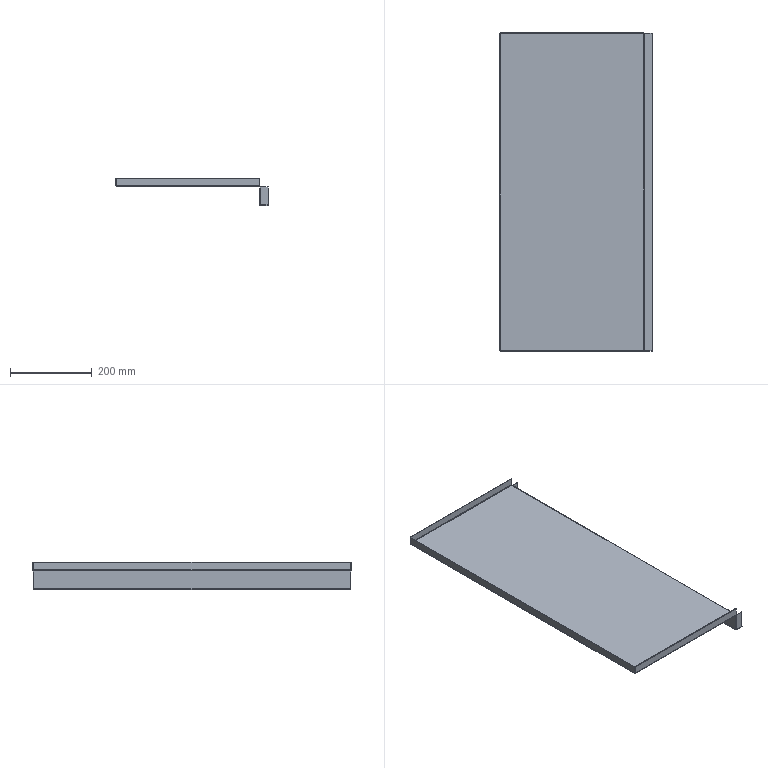Part | STEP file | X77-03014 | 1 solid | 66 faces | box 371.5 x 778 x 66 mm | volume 527186 mm3 | plane 44 | cylinder 14 | spline 8 | commonest cylinder face diameters 1.473 x7 4.473 x7